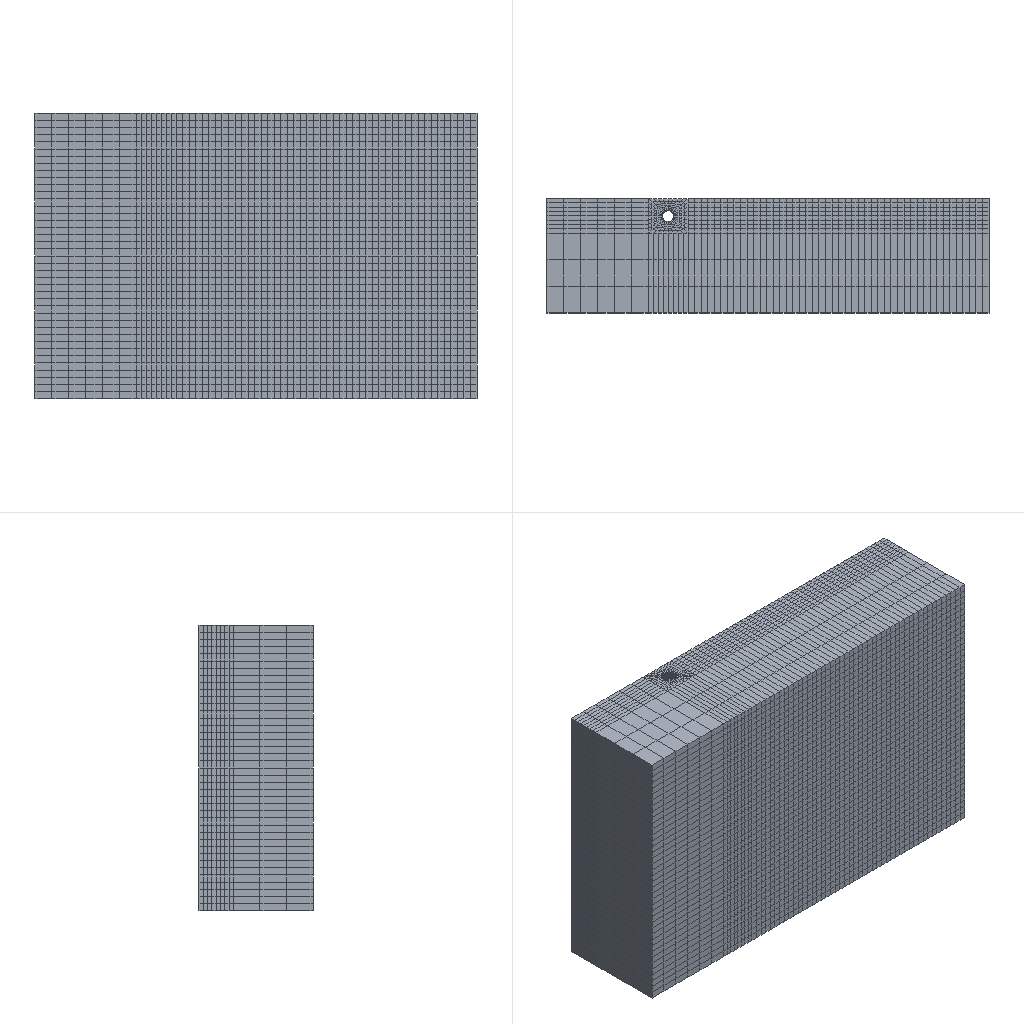Simulation study | abaqus
Set-up summary:
category,name,step,type,value,unit,region
solver,abaqus
solver,version,,,Abaqus/Explicit 6.14-4
units,not stated in the deck,,not stated
analysis,deck,,transient,transient
load_step,Step-1,Step-1,transient
load_step,Step-2,Step-2,transient
load_step,Step-3,Step-3,transient
load_step,requested,,,3
mesh,nodes,,,53202
mesh,elements,,,45388
element_type,C3D8R,,solid,40268
element_type,CIN3D8,,infinite,5120
load,load commands in deck,,count,11
bc,support commands in deck,,count,1
material,MATERIAL-GUANDAO,,in results
material,MATERIAL-TUTI,,in results
check,setup vs results,,match,"per instance, exact: element labels, types and connectivity; labels of the nodes the elements use; coordinates of those nodes at SINGLE_PRECISION in 1 of 2 instance(s)"
Abaqus input file, long lists of numbers shortened:
*Heading
** Job name: Job-22 Model name: Job-22
** Generated by: Abaqus/CAE 2020
*Preprint, echo=NO, model=NO, history=NO, contact=NO
**
** PARTS
**
*Part, name=PART-1-1
*Node
      1,   8192.395,  -941.02,       15000.
      2,   8192.395,  -941.02,        5000.
** (43612 more lines like these left out)
*Element, type=C3D8R
    1,   264,  2619, 15574,  2521,     1,    69,  1975,   155
    2,  2619,  2620, 15575, 15574,    69,    70,  1976,  1975
** (34078 more lines like these left out)
*Element, type=CIN3D8
10241,    1,  155, 2521,  264,   20,  554, 5643,  553
10242,  155,  154, 2522, 2521,  554,  555, 5644, 5643
** (4982 more lines like these left out)
*Nset, nset=_PICKEDSET14, internal, generate
     1,  43614,      1
*Elset, elset=_PICKEDSET14, internal, generate
     1,  39064,      1
** Section: Section-1-_PICKEDSET14
*Solid Section, elset=_PICKEDSET14, material=MATERIAL-TUTI
,
*End Part
**
*Part, name=PART-2-1
*Node
      1,   8201.486,  -948.852,        5000.
      2,   8201.486,  -948.852,       15000.
** (9586 more lines like these left out)
*Element, type=C3D8R
   1,  430, 2283, 6889, 2269,    1,   41, 1009,  234
   2, 2283, 2284, 6890, 6889,   41,   42, 1010, 1009
** (6186 more lines like these left out)
*Element, type=CIN3D8
6189,    2,  864, 6811,  432,   22,  886, 6829,  885
6190,  864,  863, 6812, 6811,  886,  887, 6830, 6829
** (134 more lines like these left out)
*Nset, nset=_PICKEDSET6, internal, generate
    1,  9588,     1
*Elset, elset=_PICKEDSET6, internal, generate
    1,  6324,     1
** Section: Section-2-_PICKEDSET6
*Solid Section, elset=_PICKEDSET6, material=MATERIAL-GUANDAO
,
*End Part
**
**
** ASSEMBLY
**
*Assembly, name=Assembly
**
*Instance, name=PART-1-1, part=PART-1-1
*End Instance
**
*Instance, name=PART-2-1, part=PART-2-1
*End Instance
**
*Nset, nset=_PICKEDSET182, internal, instance=PART-2-1
    1,    2,    3,    4,    5,    6,    7,    8,    9,   10,   11,   12,   13,   14,   15,   16
   17,   18,   19,   20,  131,  132,  133,  134,  135,  136,  137,  228,  229,  230,  231,  232
** (11 more lines like these left out)
*Elset, elset=_PICKEDSET182, internal, instance=PART-2-1
    1,   91,   92,  182,  183,  273,  274,  364,  365,  455,  456,  546,  547,  637,  638,  728
  729,  819,  820,  910,  911, 1001, 1002, 1092, 1093, 1183, 1184, 1274, 1275, 1365, 1366, 1456
** (15 more lines like these left out)
*Elset, elset=_SURF-1_S1, internal, instance=PART-1-1, generate
 2265,  2545,    40
*Elset, elset=_SURF-1_S3, internal, instance=PART-1-1
 12413, 12414, 12415, 12416, 12417, 12418, 20057, 20058, 20059, 20060, 20061, 20062, 20063, 20064, 20065, 20066
 20067, 20068, 20069, 20070, 20071, 20072, 20073, 20074, 20075, 20076, 20077, 20078, 20079, 20080, 20081, 20082
** (2 more lines like these left out)
*Elset, elset=_SURF-2_S1, internal, instance=PART-1-1, generate
 2265,  2545,    40
*Elset, elset=_SURF-2_S3, internal, instance=PART-1-1
 12413, 12414, 12415, 12416, 12417, 12418, 20057, 20058, 20059, 20060, 20061, 20062, 20063, 20064, 20065, 20066
 20067, 20068, 20069, 20070, 20071, 20072, 20073, 20074, 20075, 20076, 20077, 20078, 20079, 20080, 20081, 20082
** (2 more lines like these left out)
*Elset, elset=_SURF-3_S1, internal, instance=PART-1-1, generate
 2265,  2545,    40
*Elset, elset=_SURF-3_S3, internal, instance=PART-1-1
 12413, 12414, 12415, 12416, 12417, 12418, 20057, 20058, 20059, 20060, 20061, 20062, 20063, 20064, 20065, 20066
 20067, 20068, 20069, 20070, 20071, 20072, 20073, 20074, 20075, 20076, 20077, 20078, 20079, 20080, 20081, 20082
** (2 more lines like these left out)
*Elset, elset=_SURF-4_S1, internal, instance=PART-1-1, generate
 2264,  2544,    40
*Elset, elset=_SURF-4_S3, internal, instance=PART-1-1
 12461, 12462, 12463, 12464, 12465, 12466, 20425, 20426, 20427, 20428, 20429, 20430, 20431, 20432, 20433, 20434
 20435, 20436, 20437, 20438, 20439, 20440, 20441, 20442, 20443, 20444, 20445, 20446, 20447, 20448, 20449, 20450
** (2 more lines like these left out)
*Elset, elset=_SURF-5_S1, internal, instance=PART-1-1, generate
 2264,  2544,    40
*Elset, elset=_SURF-5_S3, internal, instance=PART-1-1
 12461, 12462, 12463, 12464, 12465, 12466, 20425, 20426, 20427, 20428, 20429, 20430, 20431, 20432, 20433, 20434
 20435, 20436, 20437, 20438, 20439, 20440, 20441, 20442, 20443, 20444, 20445, 20446, 20447, 20448, 20449, 20450
** (2 more lines like these left out)
*Elset, elset=_SURF-6_S1, internal, instance=PART-1-1, generate
 2256,  2536,    40
*Elset, elset=_SURF-6_S3, internal, instance=PART-1-1
 12845, 12846, 12847, 12848, 12849, 12850, 23369, 23370, 23371, 23372, 23373, 23374, 23375, 23376, 23377, 23378
 23379, 23380, 23381, 23382, 23383, 23384, 23385, 23386, 23387, 23388, 23389, 23390, 23391, 23392, 23393, 23394
** (2 more lines like these left out)
*Elset, elset=_SURF-7_S1, internal, instance=PART-1-1, generate
 2256,  2536,    40
*Elset, elset=_SURF-7_S3, internal, instance=PART-1-1
 12845, 12846, 12847, 12848, 12849, 12850, 23369, 23370, 23371, 23372, 23373, 23374, 23375, 23376, 23377, 23378
 23379, 23380, 23381, 23382, 23383, 23384, 23385, 23386, 23387, 23388, 23389, 23390, 23391, 23392, 23393, 23394
** (2 more lines like these left out)
*Elset, elset=_SURF-8_S1, internal, instance=PART-1-1, generate
 2256,  2536,    40
*Elset, elset=_SURF-8_S3, internal, instance=PART-1-1
 12845, 12846, 12847, 12848, 12849, 12850, 23369, 23370, 23371, 23372, 23373, 23374, 23375, 23376, 23377, 23378
 23379, 23380, 23381, 23382, 23383, 23384, 23385, 23386, 23387, 23388, 23389, 23390, 23391, 23392, 23393, 23394
** (2 more lines like these left out)
*Elset, elset=_SURF-9_S1, internal, instance=PART-1-1, generate
 2255,  2535,    40
*Elset, elset=_SURF-9_S3, internal, instance=PART-1-1
 12893, 12894, 12895, 12896, 12897, 12898, 23737, 23738, 23739, 23740, 23741, 23742, 23743, 23744, 23745, 23746
 23747, 23748, 23749, 23750, 23751, 23752, 23753, 23754, 23755, 23756, 23757, 23758, 23759, 23760, 23761, 23762
** (2 more lines like these left out)
*Elset, elset=_SURF-10_S1, internal, instance=PART-1-1, generate
 2255,  2535,    40
*Elset, elset=_SURF-10_S3, internal, instance=PART-1-1
 12893, 12894, 12895, 12896, 12897, 12898, 23737, 23738, 23739, 23740, 23741, 23742, 23743, 23744, 23745, 23746
 23747, 23748, 23749, 23750, 23751, 23752, 23753, 23754, 23755, 23756, 23757, 23758, 23759, 23760, 23761, 23762
** (2 more lines like these left out)
*Elset, elset=_SURF-GUANDAONEI_S2, internal, instance=PART-2-1
    1,    2,    3,    4,    5,    6,    7,    8,    9,   10,   11,   12,   13,   14,   15,   16
   17,   18,   19,   20,   21,   22,   23,   24,   25,   26,   27,   28,   29,   30,   31,   32
** (192 more lines like these left out)
*Elset, elset=_SURF-GUANDAOWAI_S1, internal, instance=PART-2-1
  729,  730,  731,  732,  733,  734,  735,  736,  737,  738,  739,  740,  741,  742,  743,  744
  745,  746,  747,  748,  749,  750,  751,  752,  753,  754,  755,  756,  757,  758,  759,  760
** (192 more lines like these left out)
*Elset, elset=_SURF-TUTINEI_S2, internal, instance=PART-1-1
    1,    2,    3,    4,    5,    6,    7,    8,    9,   10,   11,   12,   13,   14,   15,   16
   17,   18,   19,   20,   21,   22,   23,   24,   25,   26,   27,   28,   29,   30,   31,   32
** (58 more lines like these left out)
*Elset, elset=_SURF-TUTINEI_S3, internal, instance=PART-1-1
 7681, 7682, 7683, 7684, 7685, 7686, 7687, 7688, 7689, 7690, 7691, 7692, 7693, 7694, 7695, 7696
 7697, 7698, 7699, 7700, 7701, 7702, 7703, 7704, 7705, 7706, 7707, 7708, 7709, 7710, 7711, 7712
** (18 more lines like these left out)
*Elset, elset=_SURF-1_S1_1, internal, instance=PART-1-1, generate
 2265,  2545,    40
*Elset, elset=_SURF-1_S3_1, internal, instance=PART-1-1
 12413, 12414, 12415, 12416, 12417, 12418, 20057, 20058, 20059, 20060, 20061, 20062, 20063, 20064, 20065, 20066
 20067, 20068, 20069, 20070, 20071, 20072, 20073, 20074, 20075, 20076, 20077, 20078, 20079, 20080, 20081, 20082
** (2 more lines like these left out)
*Surface, type=ELEMENT, name=SURF-1
_SURF-1_S1_1, S1
_SURF-1_S3_1, S3
*Elset, elset=_SURF-2_S1_1, internal, instance=PART-1-1, generate
 2265,  2545,    40
*Elset, elset=_SURF-2_S3_1, internal, instance=PART-1-1
 12413, 12414, 12415, 12416, 12417, 12418, 20057, 20058, 20059, 20060, 20061, 20062, 20063, 20064, 20065, 20066
 20067, 20068, 20069, 20070, 20071, 20072, 20073, 20074, 20075, 20076, 20077, 20078, 20079, 20080, 20081, 20082
** (2 more lines like these left out)
*Surface, type=ELEMENT, name=SURF-2
_SURF-2_S1_1, S1
_SURF-2_S3_1, S3
*Elset, elset=_SURF-3_S1_1, internal, instance=PART-1-1, generate
 2265,  2545,    40
*Elset, elset=_SURF-3_S3_1, internal, instance=PART-1-1
 12413, 12414, 12415, 12416, 12417, 12418, 20057, 20058, 20059, 20060, 20061, 20062, 20063, 20064, 20065, 20066
 20067, 20068, 20069, 20070, 20071, 20072, 20073, 20074, 20075, 20076, 20077, 20078, 20079, 20080, 20081, 20082
** (2 more lines like these left out)
*Surface, type=ELEMENT, name=SURF-3
_SURF-3_S1_1, S1
_SURF-3_S3_1, S3
*Elset, elset=_SURF-4_S1_1, internal, instance=PART-1-1, generate
 2264,  2544,    40
*Elset, elset=_SURF-4_S3_1, internal, instance=PART-1-1
 12461, 12462, 12463, 12464, 12465, 12466, 20425, 20426, 20427, 20428, 20429, 20430, 20431, 20432, 20433, 20434
 20435, 20436, 20437, 20438, 20439, 20440, 20441, 20442, 20443, 20444, 20445, 20446, 20447, 20448, 20449, 20450
** (2 more lines like these left out)
*Surface, type=ELEMENT, name=SURF-4
_SURF-4_S1_1, S1
_SURF-4_S3_1, S3
*Elset, elset=_SURF-5_S1_1, internal, instance=PART-1-1, generate
 2264,  2544,    40
*Elset, elset=_SURF-5_S3_1, internal, instance=PART-1-1
 12461, 12462, 12463, 12464, 12465, 12466, 20425, 20426, 20427, 20428, 20429, 20430, 20431, 20432, 20433, 20434
 20435, 20436, 20437, 20438, 20439, 20440, 20441, 20442, 20443, 20444, 20445, 20446, 20447, 20448, 20449, 20450
** (2 more lines like these left out)
*Surface, type=ELEMENT, name=SURF-5
_SURF-5_S1_1, S1
_SURF-5_S3_1, S3
*Elset, elset=_SURF-6_S1_1, internal, instance=PART-1-1, generate
 2256,  2536,    40
*Elset, elset=_SURF-6_S3_1, internal, instance=PART-1-1
 12845, 12846, 12847, 12848, 12849, 12850, 23369, 23370, 23371, 23372, 23373, 23374, 23375, 23376, 23377, 23378
 23379, 23380, 23381, 23382, 23383, 23384, 23385, 23386, 23387, 23388, 23389, 23390, 23391, 23392, 23393, 23394
** (2 more lines like these left out)
*Surface, type=ELEMENT, name=SURF-6
_SURF-6_S1_1, S1
_SURF-6_S3_1, S3
*Elset, elset=_SURF-7_S1_1, internal, instance=PART-1-1, generate
 2256,  2536,    40
*Elset, elset=_SURF-7_S3_1, internal, instance=PART-1-1
 12845, 12846, 12847, 12848, 12849, 12850, 23369, 23370, 23371, 23372, 23373, 23374, 23375, 23376, 23377, 23378
 23379, 23380, 23381, 23382, 23383, 23384, 23385, 23386, 23387, 23388, 23389, 23390, 23391, 23392, 23393, 23394
** (2 more lines like these left out)
*Surface, type=ELEMENT, name=SURF-7
_SURF-7_S1_1, S1
_SURF-7_S3_1, S3
*Elset, elset=_SURF-8_S1_1, internal, instance=PART-1-1, generate
 2256,  2536,    40
*Elset, elset=_SURF-8_S3_1, internal, instance=PART-1-1
 12845, 12846, 12847, 12848, 12849, 12850, 23369, 23370, 23371, 23372, 23373, 23374, 23375, 23376, 23377, 23378
 23379, 23380, 23381, 23382, 23383, 23384, 23385, 23386, 23387, 23388, 23389, 23390, 23391, 23392, 23393, 23394
** (2 more lines like these left out)
*Surface, type=ELEMENT, name=SURF-8
_SURF-8_S1_1, S1
_SURF-8_S3_1, S3
*Elset, elset=_SURF-9_S1_1, internal, instance=PART-1-1, generate
 2255,  2535,    40
*Elset, elset=_SURF-9_S3_1, internal, instance=PART-1-1
 12893, 12894, 12895, 12896, 12897, 12898, 23737, 23738, 23739, 23740, 23741, 23742, 23743, 23744, 23745, 23746
 23747, 23748, 23749, 23750, 23751, 23752, 23753, 23754, 23755, 23756, 23757, 23758, 23759, 23760, 23761, 23762
** (2 more lines like these left out)
*Surface, type=ELEMENT, name=SURF-9
_SURF-9_S1_1, S1
_SURF-9_S3_1, S3
*Elset, elset=_SURF-10_S1_1, internal, instance=PART-1-1, generate
 2255,  2535,    40
*Elset, elset=_SURF-10_S3_1, internal, instance=PART-1-1
 12893, 12894, 12895, 12896, 12897, 12898, 23737, 23738, 23739, 23740, 23741, 23742, 23743, 23744, 23745, 23746
 23747, 23748, 23749, 23750, 23751, 23752, 23753, 23754, 23755, 23756, 23757, 23758, 23759, 23760, 23761, 23762
** (2 more lines like these left out)
*Surface, type=ELEMENT, name=SURF-10
_SURF-10_S1_1, S1
_SURF-10_S3_1, S3
*Surface, type=ELEMENT, name=SURF-GUANDAONEI
_SURF-GUANDAONEI_S2, S2
*Surface, type=ELEMENT, name=SURF-GUANDAOWAI
_SURF-GUANDAOWAI_S1, S1
*Elset, elset=_SURF-TUTINEI_S2_1, internal, instance=PART-1-1
    1,    2,    3,    4,    5,    6,    7,    8,    9,   10,   11,   12,   13,   14,   15,   16
   17,   18,   19,   20,   21,   22,   23,   24,   25,   26,   27,   28,   29,   30,   31,   32
** (58 more lines like these left out)
*Elset, elset=_SURF-TUTINEI_S3_1, internal, instance=PART-1-1
 7681, 7682, 7683, 7684, 7685, 7686, 7687, 7688, 7689, 7690, 7691, 7692, 7693, 7694, 7695, 7696
 7697, 7698, 7699, 7700, 7701, 7702, 7703, 7704, 7705, 7706, 7707, 7708, 7709, 7710, 7711, 7712
** (18 more lines like these left out)
*Surface, type=ELEMENT, name=SURF-TUTINEI
_SURF-TUTINEI_S2_1, S2
_SURF-TUTINEI_S3_1, S3
** Constraint: CONSTRAINT-1-1
*Tie, name=CONSTRAINT-1-1, adjust=yes
SURF-GUANDAOWAI, SURF-TUTINEI
*End Assembly
*Amplitude, name=AMP-1
           0.07,     0.5411,            0.14,     0.4955,            0.21,     0.5072,            0.28,     0.5991
           0.35,     0.6713,            0.42,     0.6774,            0.49,     0.5947,            0.56,     0.5263
           0.63,     0.5566,             0.7,     0.5985,            0.77,     0.5476,            0.84,     0.4736
           0.91,     0.5199,            0.98,     0.5887,            1.05,     0.6221,            1.12,     0.6117
           1.19,        0.574,            1.26,     0.6128,            1.33,     0.6529,             1.4,     0.5639
           1.47,     0.4659,            1.54,     0.528,            1.61,     0.6547,            1.68,     0.6567
           1.75,     0.6037,            1.82,     0.6075,            1.89,     0.6134,            1.96,     0.5673
           2.03,     0.499,             2.1,     0.5092,            2.17,     0.5867,            2.24,     0.5149
           2.31,     0.4364,            2.38,     0.5068,            2.45,     0.5874,            2.52,     0.5768
           2.59,     0.5433,            2.66,     0.4688,            2.73,     0.5038,             2.8,     0.5647
           2.87,     0.6048,            2.94,       0.6065,            3.01,     0.5944,            3.08,     0.5507
           3.15,     0.5688,            3.22,     0.5457,            3.29,     0.5195,            3.36,       0.6003
           3.43,     0.7116,             3.5,     0.6556,            3.57,     0.5233,            3.64,     0.5312
           3.71,     0.5478,            3.78,     0.5253,            3.85,     0.5845,            3.92,     0.6598
           3.99,     0.568,            4.06,     0.4078,            4.13,     0.4899,             4.2,     0.6071
*Amplitude, name=AMP-2
           0.07,     0.6412,            0.14,     0.5919,            0.21,     0.4852,            0.28,     0.5071
           0.35,     0.5575,            0.42,     0.5505,            0.49,     0.537,            0.56,       0.5474
           0.63,     0.5998,             0.7,     0.6222,            0.77,     0.6254,            0.84,     0.6583
           0.91,     0.6364,            0.98,     0.5416,            1.05,     0.524,            1.12,     0.5751
           1.19,     0.6039,            1.26,     0.5919,            1.33,      0.5643,             1.4,     0.5625
           1.47,     0.5803,            1.54,     0.5566,            1.61,     0.5337,            1.68,     0.5568
           1.75,     0.5865,            1.82,     0.5703,            1.89,     0.5635,            1.96,     0.5828
           2.03,     0.6388,             2.1,        0.7294,            2.17,     0.714,            2.24,     0.5569
           2.31,     0.4335,            2.38,     0.5799,            2.45,     0.6909,            2.52,     0.6735
           2.59,     0.6237,            2.66,     0.6025,            2.73,     0.6137,             2.8,     0.6429
           2.87,     0.6655,            2.94,     0.6448,            3.01,     0.5669,            3.08,       0.4776
           3.15,     0.4348,            3.22,      0.439,            3.29,      0.4397,            3.36,     0.5135
           3.43,     0.6049,             3.5,     0.6752,            3.57,      0.7432,            3.64,     0.7719
           3.71,     0.729,            3.78,     0.6367,            3.85,     0.5479,            3.92,     0.4715
           3.99,     0.4822,            4.06,     0.5139,            4.13,      0.5902,             4.2,      0.6839
*Amplitude, name=AMP-3
           0.07,     0.5287,            0.14,      0.4465,            0.21,     0.5426,            0.28,     0.6805
           0.35,        0.7122,            0.42,     0.5948,            0.49,     0.4684,            0.56,     0.5074
           0.63,     0.5524,             0.7,     0.5278,            0.77,     0.5002,            0.84,     0.5012
           0.91,     0.5305,            0.98,     0.5407,            1.05,     0.5645,            1.12,     0.6485
           1.19,     0.6782,            1.26,     0.632,            1.33,     0.663,             1.4,     0.712
           1.47,     0.7015,            1.54,         0.6286,            1.61,     0.5666,            1.68,     0.596
           1.75,       0.6292,            1.82,      0.5933,            1.89,     0.5556,            1.96,     0.5798
           2.03,     0.5993,             2.1,     0.5581,            2.17,      0.5201,            2.24,     0.5344
           2.31,      0.6256,            2.38,     0.7246,            2.45,     0.6739,            2.52,      0.515
           2.59,     0.4748,            2.66,     0.6828,            2.73,     0.7779,             2.8,      0.7083
           2.87,     0.6004,            2.94,     0.5569,            3.01,     0.5781,            3.08,     0.6557
           3.15,     0.7352,            3.22,     0.7385,            3.29,     0.6511,            3.36,     0.5352
           3.43,     0.4819,             3.5,     0.4907,            3.57,     0.5138,            3.64,     0.5703
           3.71,     0.6029,            3.78,     0.6086,            3.85,     0.6394,            3.92,     0.6798
           3.99,     0.6986,            4.06,     0.6723,            4.13,     0.6181,             4.2,     0.5406
*Amplitude, name=AMP-4
           0.07,     0.476,            0.14,     0.4126,            0.21,      0.564,            0.28,     0.6839
           0.35,     0.6876,            0.42,     0.6614,            0.49,     0.6682,            0.56,     0.722
           0.63,     0.7573,             0.7,     0.7147,            0.77,     0.6979,            0.84,     0.5891
           0.91,     0.4386,            0.98,     0.3825,            1.05,     0.4151,            1.12,     0.4533
           1.19,     0.4849,            1.26,     0.4671,            1.33,     0.4856,             1.4,     0.5578
           1.47,      0.6068,            1.54,     0.6038,            1.61,     0.5877,            1.68,     0.6113
           1.75,     0.6134,            1.82,     0.6376,            1.89,     0.6522,            1.96,     0.6554
           2.03,     0.7302,             2.1,      0.6907,            2.17,     0.4926,            2.24,     0.3662
           2.31,     0.4592,            2.38,     0.6015,            2.45,     0.5837,            2.52,     0.5128
           2.59,      0.5321,            2.66,     0.5948,            2.73,     0.6032,             2.8,     0.5318
           2.87,     0.4952,            2.94,       0.5675,            3.01,       0.5225,            3.08,     0.4817
           3.15,     0.5215,            3.22,     0.5387,            3.29,     0.5494,            3.36,     0.635
           3.43,     0.6229,             3.5,     0.6631,            3.57,     0.6493,            3.64,     0.5794
           3.71,     0.5434,            3.78,     0.5361,            3.85,     0.4992,            3.92,     0.5933
           3.99,      0.6021,            4.06,     0.4941,            4.13,     0.4959,             4.2,       0.5924
*Amplitude, name=AMP-5
           0.07,     0.491,            0.14,     0.5854,            0.21,     0.8102,            0.28,     0.7681
           0.35,     0.5398,            0.42,     0.4474,            0.49,       0.5891,            0.56,     0.6884
           0.63,     0.6827,             0.7,     0.639,            0.77,     0.6255,            0.84,     0.657
           0.91,     0.6589,            0.98,     0.617,            1.05,     0.6312,            1.12,     0.5654
           1.19,     0.4802,            1.26,     0.4883,            1.33,     0.5611,             1.4,     0.6043
           1.47,     0.5976,            1.54,       0.5255,            1.61,     0.5169,            1.68,     0.6062
           1.75,     0.6653,            1.82,       0.6422,            1.89,     0.6123,            1.96,     0.6206
           2.03,     0.6114,             2.1,     0.6053,            2.17,     0.5755,            2.24,     0.5828
           2.31,     0.7067,            2.38,         0.6598,            2.45,     0.4521,            2.52,      0.3531
           2.59,     0.5301,            2.66,     0.7135,            2.73,     0.6765,             2.8,     0.5671
           2.87,     0.523,            2.94,     0.5488,            3.01,     0.5563,            3.08,     0.5287
           3.15,     0.5691,            3.22,     0.6729,            3.29,      0.6115,            3.36,     0.5628
           3.43,     0.5757,             3.5,         0.5976,            3.57,     0.6396,            3.64,     0.6924
           3.71,        0.6154,            3.78,     0.5941,            3.85,      0.5289,            3.92,     0.4767
           3.99,     0.5101,            4.06,     0.5661,            4.13,     0.5775,             4.2,     0.6634
*Amplitude, name=AMP-6
           0.07,     0.498,            0.14,     0.4831,            0.21,      0.5476,            0.28,     0.6264
           0.35,      0.6356,            0.42,       0.6003,            0.49,     0.5461,            0.56,      0.5107
           0.63,     0.5489,             0.7,     0.6058,            0.77,     0.557,            0.84,     0.4797
           0.91,        0.5473,            0.98,     0.6532,            1.05,      0.6829,            1.12,     0.6386
           1.19,     0.5511,            1.26,     0.5119,            1.33,      0.5649,             1.4,     0.5882
           1.47,     0.5825,            1.54,     0.597,            1.61,     0.5801,            1.68,     0.4994
           1.75,     0.4833,            1.82,     0.5753,            1.89,     0.6372,            1.96,     0.6042
           2.03,     0.5305,             2.1,        0.5237,            2.17,     0.5985,            2.24,     0.6035
           2.31,     0.5515,            2.38,     0.6251,            2.45,     0.7359,            2.52,     0.7316
           2.59,     0.6419,            2.66,     0.564,            2.73,     0.5313,             2.8,     0.5142
           2.87,     0.5597,            2.94,     0.5628,            3.01,     0.5595,            3.08,     0.6121
           3.15,      0.66,            3.22,     0.579,            3.29,     0.4467,            3.36,      0.5043
           3.43,      0.6312,             3.5,     0.6419,            3.57,     0.5811,            3.64,     0.5593
           3.71,      0.5255,            3.78,         0.4862,            3.85,      0.5491,            3.92,     0.6607
           3.99,     0.6297,            4.06,     0.5139,            4.13,     0.5281,             4.2,     0.6196
*Amplitude, name=AMP-7
           0.07,     0.6201,            0.14,     0.7353,            0.21,     0.7553,            0.28,     0.6318
           0.35,     0.5231,            0.42,     0.5277,            0.49,     0.5392,            0.56,     0.6058
           0.63,     0.7139,             0.7,     0.6806,            0.77,     0.5281,            0.84,     0.436
           0.91,     0.5114,            0.98,     0.592,            1.05,     0.5894,            1.12,      0.5396
           1.19,     0.5563,            1.26,     0.5515,            1.33,     0.567,             1.4,     0.6917
           1.47,     0.7275,            1.54,     0.6309,            1.61,     0.5457,            1.68,     0.5034
           1.75,     0.4461,            1.82,       0.4586,            1.89,     0.4608,            1.96,     0.4533
           2.03,     0.5416,             2.1,     0.6014,            2.17,       0.5953,            2.24,     0.6055
           2.31,     0.5755,            2.38,     0.4993,            2.45,     0.4771,            2.52,     0.5945
           2.59,     0.6543,            2.66,     0.5982,            2.73,     0.5254,             2.8,     0.5107
           2.87,      0.5793,            2.94,     0.6174,            3.01,     0.5515,            3.08,     0.4833
           3.15,     0.5835,            3.22,     0.7147,            3.29,     0.7526,            3.36,     0.789
           3.43,     0.7787,             3.5,     0.6874,            3.57,     0.6024,            3.64,     0.5191
           3.71,     0.4362,            3.78,     0.5116,            3.85,     0.6993,            3.92,     0.7072
           3.99,     0.5132,            4.06,     0.3709,            4.13,     0.5578,             4.2,     0.6998
*Amplitude, name=AMP-8
           0.07,     0.5598,            0.14,     0.5164,            0.21,     0.5614,            0.28,     0.5829
           0.35,     0.6393,            0.42,     0.7276,            0.49,     0.7092,            0.56,     0.5716
           0.63,     0.484,             0.7,     0.5147,            0.77,     0.5507,            0.84,     0.6557
           0.91,     0.749,            0.98,     0.6771,            1.05,     0.5121,            1.12,     0.4579
           1.19,     0.5913,            1.26,          0.6919,            1.33,     0.6773,             1.4,     0.6186
           1.47,     0.5937,            1.54,     0.5275,            1.61,     0.5317,            1.68,     0.7001
           1.75,     0.7479,            1.82,      0.6503,            1.89,     0.5756,            1.96,     0.5437
           2.03,     0.5092,             2.1,     0.527,            2.17,     0.4932,            2.24,     0.4671
           2.31,     0.5591,            2.38,      0.6036,            2.45,     0.5734,            2.52,     0.5718
           2.59,     0.5441,            2.66,      0.4813,            2.73,     0.4766,             2.8,     0.5919
           2.87,     0.629,            2.94,     0.5715,            3.01,     0.528,            3.08,      0.5559
           3.15,     0.6651,            3.22,     0.7034,            3.29,     0.6071,            3.36,     0.5193
           3.43,     0.6156,             3.5,     0.7416,            3.57,     0.7846,            3.64,      0.7975
           3.71,     0.7356,            3.78,     0.6073,            3.85,       0.5213,            3.92,     0.4678
           3.99,      0.4637,            4.06,     0.6327,            4.13,     0.8168,             4.2,      0.7672
*Amplitude, name=AMP-9
           0.07,     0.6106,            0.14,     0.6084,            0.21,     0.6391,            0.28,     0.6328
           0.35,     0.566,            0.42,     0.5305,            0.49,     0.531,            0.56,     0.5261
           0.63,     0.5589,             0.7,     0.604,            0.77,     0.604,            0.84,     0.5559
           0.91,        0.5311,            0.98,     0.5472,            1.05,     0.5823,            1.12,         0.6072
           1.19,     0.6091,            1.26,     0.6292,            1.33,     0.6093,             1.4,     0.5651
           1.47,     0.5888,            1.54,     0.5683,            1.61,     0.5092,            1.68,     0.5549
           1.75,     0.641,            1.82,     0.6061,            1.89,     0.5728,            1.96,       0.5762
           2.03,     0.5731,             2.1,     0.621,            2.17,     0.6547,            2.24,      0.6487
           2.31,     0.6743,            2.38,      0.7184,            2.45,     0.6771,            2.52,      0.5658
           2.59,     0.5646,            2.66,     0.638,            2.73,     0.6492,             2.8,      0.5664
           2.87,         0.4564,            2.94,     0.4857,            3.01,     0.5407,            3.08,     0.5053
           3.15,     0.5035,            3.22,      0.5549,            3.29,     0.559,            3.36,     0.5386
           3.43,     0.5632,             3.5,      0.5727,            3.57,     0.5394,            3.64,     0.564
           3.71,     0.5554,            3.78,     0.4808,            3.85,     0.4707,            3.92,     0.56
           3.99,     0.5858,            4.06,     0.4973,            4.13,     0.4251,             4.2,      0.5327
*Amplitude, name=AMP-10
           0.07,     0.576,            0.14,     0.5414,            0.21,      0.5965,            0.28,     0.6274
           0.35,     0.5939,            0.42,     0.5833,            0.49,     0.5993,            0.56,      0.581
           0.63,     0.5193,             0.7,      0.5147,            0.77,     0.5533,            0.84,     0.5731
           0.91,     0.6062,            0.98,     0.622,            1.05,     0.6019,            1.12,     0.5725
           1.19,     0.5987,            1.26,     0.6397,            1.33,     0.6772,             1.4,     0.6715
           1.47,     0.6275,            1.54,     0.5838,            1.61,     0.5376,            1.68,     0.5459
           1.75,     0.6156,            1.82,      0.5948,            1.89,     0.5429,            1.96,     0.6295
           2.03,     0.7236,             2.1,     0.6935,            2.17,      0.6466,            2.24,     0.62
           2.31,      0.6026,            2.38,     0.642,            2.45,     0.643,            2.52,     0.6157
           2.59,     0.645,            2.66,     0.6897,            2.73,     0.63,             2.8,      0.5249
           2.87,     0.5463,            2.94,     0.637,            3.01,     0.6635,            3.08,     0.5951
           3.15,     0.5371,            3.22,     0.5802,            3.29,     0.601,            3.36,     0.5284
           3.43,       0.5122,             3.5,     0.5722,            3.57,      0.5739,            3.64,     0.5394
           3.71,     0.5255,            3.78,     0.5057,            3.85,     0.4685,            3.92,     0.5417
           3.99,     0.5983,            4.06,       0.5902,            4.13,     0.5922,             4.2,     0.6379
**
** MATERIALS
**
*Material, name=MATERIAL-GUANDAO
*Density
 7.85e-09,
*Elastic
210000., 0.3
*Material, name=MATERIAL-TUTI
*Density
 1.78e-09,
*Drucker Prager
36.,1.,0.
*Drucker Prager Hardening
 0.17,    0.
 0.65, 0.035
 0.75, 0.051
  0.8, 0.073
 0.85, 0.092
*Elastic
 14.4, 0.4
**
** INTERACTION PROPERTIES
**
*Surface Interaction, name=INTPROP-1
*Friction
 0.4,
*Surface Behavior, pressure-overclosure=HARD
** ----------------------------------------------------------------
**
** STEP: Step-1
**
*Step, name=Step-1, nlgeom=YES
*Dynamic, Explicit
, 1.
*Bulk Viscosity
0.06, 1.2
**
** LOADS
**
** Name: SURFFORCE-1   Type: Pressure
*Dsload
SURF-GUANDAONEI, PNU, 6.
**
** OUTPUT REQUESTS
**
*Restart, write, number interval=1, time marks=NO
**
** FIELD OUTPUT: F-Output-1
**
*Output, field, variable=PRESELECT, number interval=10
**
** HISTORY OUTPUT: H-Output-1
**
*Output, history, variable=PRESELECT, time interval=0.1
*End Step
** ----------------------------------------------------------------
**
** STEP: Step-2
**
*Step, name=Step-2, nlgeom=YES
*Dynamic, Explicit
, 1.
*Bulk Viscosity
0.06, 1.2
**
** OUTPUT REQUESTS
**
*Restart, write, number interval=1, time marks=NO
**
** FIELD OUTPUT: F-Output-2
**
*Output, field, variable=PRESELECT, number interval=10
**
** HISTORY OUTPUT: H-Output-2
**
*Output, history, variable=PRESELECT, time interval=0.1
*End Step
** ----------------------------------------------------------------
**
** STEP: Step-3
**
*Step, name=Step-3, nlgeom=YES
*Dynamic, Explicit
, 3.
*Bulk Viscosity
0.06, 1.2
**
** BOUNDARY CONDITIONS
**
** Name: Disp-BC-1 Type: 对称/反对称/完全固定
*Boundary
_PICKEDSET182, PINNED
**
** LOADS
**
** Name: SURFFORCE-2   Type: Pressure
*Dsload, amplitude=AMP-1
SURF-1, PNU, 1.
** Name: SURFFORCE-3   Type: Pressure
*Dsload, amplitude=AMP-2
SURF-2, PNU, 1.
** Name: SURFFORCE-4   Type: Pressure
*Dsload, amplitude=AMP-3
SURF-4, PNU, 1.
** Name: SURFFORCE-5   Type: Pressure
*Dsload, amplitude=AMP-4
SURF-3, PNU, 1.
** Name: SURFFORCE-6   Type: Pressure
*Dsload, amplitude=AMP-5
SURF-5, PNU, 1.
** Name: SURFFORCE-7   Type: Pressure
*Dsload, amplitude=AMP-6
SURF-6, PNU, 1.
** Name: SURFFORCE-8   Type: Pressure
*Dsload, amplitude=AMP-7
SURF-7, PNU, 1.
** Name: SURFFORCE-9   Type: Pressure
*Dsload, amplitude=AMP-8
SURF-9, PNU, 1.
** Name: SURFFORCE-10   Type: Pressure
*Dsload, amplitude=AMP-9
SURF-8, PNU, 1.
** Name: SURFFORCE-11   Type: Pressure
*Dsload, amplitude=AMP-10
SURF-10, PNU, 1.
**
** INTERACTIONS
**
** Interaction: INT-1-1
*Contact Pair, interaction=INTPROP-1, mechanical constraint=KINEMATIC, cpset=INT-1-1
SURF-GUANDAOWAI, SURF-TUTINEI
**
** OUTPUT REQUESTS
**
*Restart, write, number interval=1, time marks=NO
**
** FIELD OUTPUT: F-Output-3
**
*Output, field, variable=PRESELECT, number interval=60
**
** HISTORY OUTPUT: H-Output-3
**
*Output, history, variable=PRESELECT, time interval=0.05
*End Step
Results summary:
result,step,Step-1,completed,increments=1711205 time=1.0/1.0
result,step,Step-2,completed,increments=1711205 time=1.0/1.0
result,step,Step-3,completed,increments=5486077 time=3.0/3.0
result,analysis,,,transient
result,last_loadstep,,,3
result,primary field,,,U
result,reaction total,,FX,-37367.673,model units
result,reaction total,,FY,299886.962,model units
result,reaction total,,FZ,-84949.882,model units